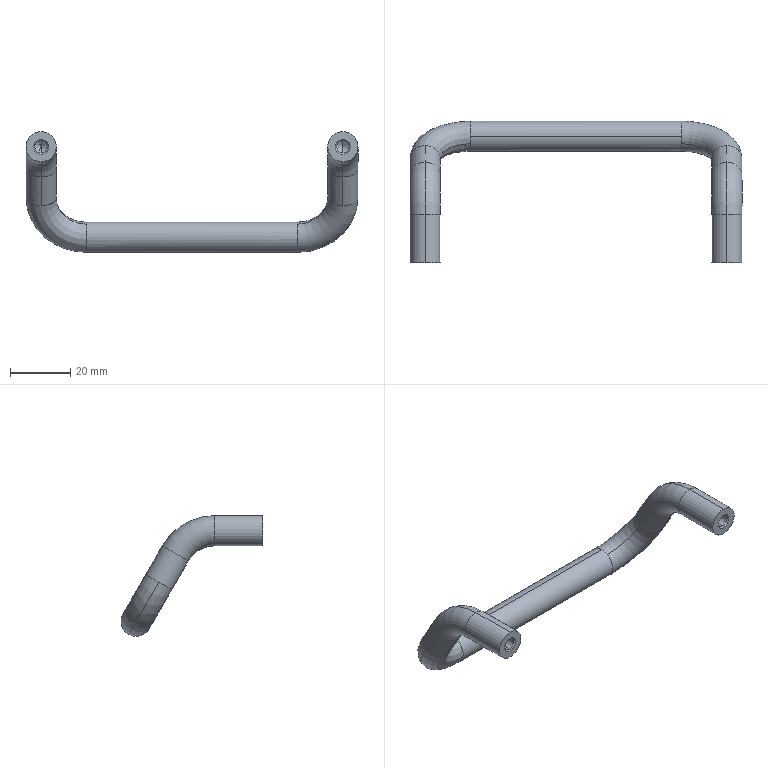Part | SolidWorks | features BaseBody 1 | 1 solid | 39 faces | box 110 x 47 x 40 mm | volume 15475 mm3 | cylinder 14 | plane 9 | cone 8 | torus 6 | spline 2 | commonest cylinder face diameters 10 x6 4.134 x4 9.998 x4